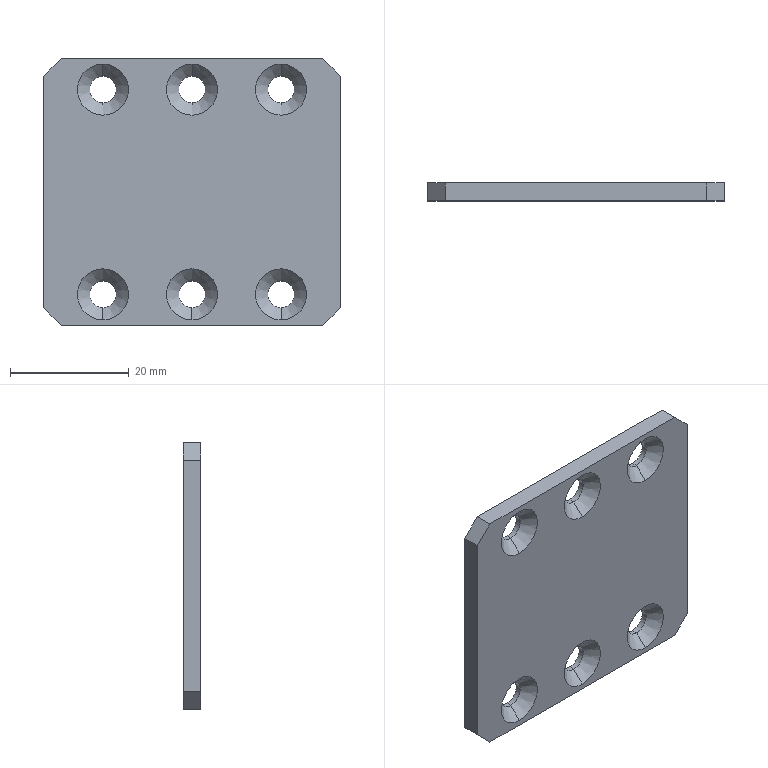Part | SolidWorks | features Chamfer 1, Extrusion 1, HoleWzd 1 | 1 solid | 34 faces | box 50 x 3 x 45 mm | volume 6177 mm3 | cone 12 | cylinder 12 | plane 10 | commonest cylinder face diameters 4.5 x12
STEP:
#1=CARTESIAN_POINT('',(-15.,2.05,-15.));
#2=VERTEX_POINT('',#1);
#3=CARTESIAN_POINT('',(-15.,2.05,-19.5));
#4=VERTEX_POINT('',#3);
#5=CARTESIAN_POINT('',(-15.,2.05,-17.25));
#6=DIRECTION('',(0.,-1.,0.));
#7=DIRECTION('',(0.,0.,-1.));
#8=AXIS2_PLACEMENT_3D('',#5,#6,#7);
#9=CIRCLE('',#8,2.25);
#10=EDGE_CURVE('',#2,#4,#9,.T.);
#11=ORIENTED_EDGE('',*,*,#10,.F.);
#12=CARTESIAN_POINT('',(-15.,0.,-12.95));
#13=VERTEX_POINT('',#12);
#14=CARTESIAN_POINT('',(-15.,0.,-12.95));
#15=DIRECTION('',(0.,-0.7071,0.7071));
#16=VECTOR('',#15,1000.);
#17=LINE('',#14,#16);
#18=EDGE_CURVE('',#2,#13,#17,.T.);
#19=ORIENTED_EDGE('',*,*,#18,.T.);
#20=CARTESIAN_POINT('',(-15.,0.,-21.55));
#21=VERTEX_POINT('',#20);
#22=CARTESIAN_POINT('',(-15.,0.,-17.25));
#23=DIRECTION('',(0.,-1.,0.));
#24=DIRECTION('',(0.,0.,-1.));
#25=AXIS2_PLACEMENT_3D('',#22,#23,#24);
#26=CIRCLE('',#25,4.3);
#27=EDGE_CURVE('',#13,#21,#26,.T.);
#28=ORIENTED_EDGE('',*,*,#27,.T.);
#29=CARTESIAN_POINT('',(-15.,0.,-21.55));
#30=DIRECTION('',(0.,-0.7071,-0.7071));
#31=VECTOR('',#30,1000.);
#32=LINE('',#29,#31);
#33=EDGE_CURVE('',#4,#21,#32,.T.);
#34=ORIENTED_EDGE('',*,*,#33,.F.);
#35=EDGE_LOOP('',(#11,#19,#28,#34));
#36=FACE_OUTER_BOUND('',#35,.T.);
#37=CARTESIAN_POINT('',(-15.,0.,-17.25));
#38=DIRECTION('',(0.,-1.,0.));
#39=DIRECTION('',(0.,0.,-1.));
#40=AXIS2_PLACEMENT_3D('',#37,#38,#39);
#41=CONICAL_SURFACE('',#40,4.3,0.7854);
#42=ADVANCED_FACE('',(#36),#41,.F.);
#43=CARTESIAN_POINT('',(-15.,3.,-19.5));
#44=VERTEX_POINT('',#43);
#45=CARTESIAN_POINT('',(-15.,3.,-15.));
#46=VERTEX_POINT('',#45);
#47=CARTESIAN_POINT('',(-15.,3.,-17.25));
#48=DIRECTION('',(0.,1.,0.));
#49=DIRECTION('',(0.,0.,1.));
#50=AXIS2_PLACEMENT_3D('',#47,#48,#49);
#51=CIRCLE('',#50,2.25);
#52=EDGE_CURVE('',#44,#46,#51,.T.);
#53=ORIENTED_EDGE('',*,*,#52,.T.);
#54=CARTESIAN_POINT('',(-15.,0.,-15.));
#55=DIRECTION('',(0.,-1.,0.));
#56=VECTOR('',#55,1000.);
#57=LINE('',#54,#56);
#58=EDGE_CURVE('',#46,#2,#57,.T.);
#59=ORIENTED_EDGE('',*,*,#58,.T.);
#60=ORIENTED_EDGE('',*,*,#10,.T.);
#61=CARTESIAN_POINT('',(-15.,0.,-19.5));
#62=DIRECTION('',(0.,-1.,0.));
#63=VECTOR('',#62,1000.);
#64=LINE('',#61,#63);
#65=EDGE_CURVE('',#44,#4,#64,.T.);
#66=ORIENTED_EDGE('',*,*,#65,.F.);
#67=EDGE_LOOP('',(#53,#59,#60,#66));
#68=FACE_OUTER_BOUND('',#67,.T.);
#69=CARTESIAN_POINT('',(-15.,0.,-17.25));
#70=DIRECTION('',(0.,-1.,0.));
#71=DIRECTION('',(0.,0.,-1.));
#72=AXIS2_PLACEMENT_3D('',#69,#70,#71);
#73=CYLINDRICAL_SURFACE('',#72,2.25);
#74=ADVANCED_FACE('',(#68),#73,.F.);
#75=CARTESIAN_POINT('',(0.,2.05,-15.));
#76=VERTEX_POINT('',#75);
#77=CARTESIAN_POINT('',(0.,2.05,-19.5));
#78=VERTEX_POINT('',#77);
#79=CARTESIAN_POINT('',(0.,2.05,-17.25));
#80=DIRECTION('',(0.,-1.,0.));
#81=DIRECTION('',(0.,0.,-1.));
#82=AXIS2_PLACEMENT_3D('',#79,#80,#81);
#83=CIRCLE('',#82,2.25);
#84=EDGE_CURVE('',#76,#78,#83,.T.);
#85=ORIENTED_EDGE('',*,*,#84,.F.);
#86=CARTESIAN_POINT('',(0.,0.,-12.95));
#87=VERTEX_POINT('',#86);
#88=CARTESIAN_POINT('',(0.,0.,-12.95));
#89=DIRECTION('',(0.,-0.7071,0.7071));
#90=VECTOR('',#89,1000.);
#91=LINE('',#88,#90);
#92=EDGE_CURVE('',#76,#87,#91,.T.);
#93=ORIENTED_EDGE('',*,*,#92,.T.);
#94=CARTESIAN_POINT('',(0.,0.,-21.55));
#95=VERTEX_POINT('',#94);
#96=CARTESIAN_POINT('',(0.,0.,-17.25));
#97=DIRECTION('',(0.,-1.,0.));
#98=DIRECTION('',(0.,0.,-1.));
#99=AXIS2_PLACEMENT_3D('',#96,#97,#98);
#100=CIRCLE('',#99,4.3);
#101=EDGE_CURVE('',#87,#95,#100,.T.);
#102=ORIENTED_EDGE('',*,*,#101,.T.);
#103=CARTESIAN_POINT('',(0.,0.,-21.55));
#104=DIRECTION('',(0.,-0.7071,-0.7071));
#105=VECTOR('',#104,1000.);
#106=LINE('',#103,#105);
#107=EDGE_CURVE('',#78,#95,#106,.T.);
#108=ORIENTED_EDGE('',*,*,#107,.F.);
#109=EDGE_LOOP('',(#85,#93,#102,#108));
#110=FACE_OUTER_BOUND('',#109,.T.);
#111=CARTESIAN_POINT('',(0.,0.,-17.25));
#112=DIRECTION('',(0.,-1.,0.));
#113=DIRECTION('',(0.,0.,-1.));
#114=AXIS2_PLACEMENT_3D('',#111,#112,#113);
#115=CONICAL_SURFACE('',#114,4.3,0.7854);
#116=ADVANCED_FACE('',(#110),#115,.F.);
#117=CARTESIAN_POINT('',(0.,3.,-19.5));
#118=VERTEX_POINT('',#117);
#119=CARTESIAN_POINT('',(0.,3.,-15.));
#120=VERTEX_POINT('',#119);
#121=CARTESIAN_POINT('',(0.,3.,-17.25));
#122=DIRECTION('',(0.,1.,0.));
#123=DIRECTION('',(0.,0.,1.));
#124=AXIS2_PLACEMENT_3D('',#121,#122,#123);
#125=CIRCLE('',#124,2.25);
#126=EDGE_CURVE('',#118,#120,#125,.T.);
#127=ORIENTED_EDGE('',*,*,#126,.T.);
#128=CARTESIAN_POINT('',(0.,0.,-15.));
#129=DIRECTION('',(0.,-1.,0.));
#130=VECTOR('',#129,1000.);
#131=LINE('',#128,#130);
#132=EDGE_CURVE('',#120,#76,#131,.T.);
#133=ORIENTED_EDGE('',*,*,#132,.T.);
#134=ORIENTED_EDGE('',*,*,#84,.T.);
#135=CARTESIAN_POINT('',(0.,0.,-19.5));
#136=DIRECTION('',(0.,-1.,0.));
#137=VECTOR('',#136,1000.);
#138=LINE('',#135,#137);
#139=EDGE_CURVE('',#118,#78,#138,.T.);
#140=ORIENTED_EDGE('',*,*,#139,.F.);
#141=EDGE_LOOP('',(#127,#133,#134,#140));
#142=FACE_OUTER_BOUND('',#141,.T.);
#143=CARTESIAN_POINT('',(0.,0.,-17.25));
#144=DIRECTION('',(0.,-1.,0.));
#145=DIRECTION('',(0.,0.,-1.));
#146=AXIS2_PLACEMENT_3D('',#143,#144,#145);
#147=CYLINDRICAL_SURFACE('',#146,2.25);
#148=ADVANCED_FACE('',(#142),#147,.F.);
#149=CARTESIAN_POINT('',(15.,2.05,-15.));
#150=VERTEX_POINT('',#149);
#151=CARTESIAN_POINT('',(15.,2.05,-19.5));
#152=VERTEX_POINT('',#151);
#153=CARTESIAN_POINT('',(15.,2.05,-17.25));
#154=DIRECTION('',(0.,-1.,0.));
#155=DIRECTION('',(0.,0.,-1.));
#156=AXIS2_PLACEMENT_3D('',#153,#154,#155);
#157=CIRCLE('',#156,2.25);
#158=EDGE_CURVE('',#150,#152,#157,.T.);
#159=ORIENTED_EDGE('',*,*,#158,.F.);
#160=CARTESIAN_POINT('',(15.,0.,-12.95));
#161=VERTEX_POINT('',#160);
#162=CARTESIAN_POINT('',(15.,0.,-12.95));
#163=DIRECTION('',(0.,-0.7071,0.7071));
#164=VECTOR('',#163,1000.);
#165=LINE('',#162,#164);
#166=EDGE_CURVE('',#150,#161,#165,.T.);
#167=ORIENTED_EDGE('',*,*,#166,.T.);
#168=CARTESIAN_POINT('',(15.,0.,-21.55));
#169=VERTEX_POINT('',#168);
#170=CARTESIAN_POINT('',(15.,0.,-17.25));
#171=DIRECTION('',(0.,-1.,0.));
#172=DIRECTION('',(0.,0.,-1.));
#173=AXIS2_PLACEMENT_3D('',#170,#171,#172);
#174=CIRCLE('',#173,4.3);
#175=EDGE_CURVE('',#161,#169,#174,.T.);
#176=ORIENTED_EDGE('',*,*,#175,.T.);
#177=CARTESIAN_POINT('',(15.,0.,-21.55));
#178=DIRECTION('',(0.,-0.7071,-0.7071));
#179=VECTOR('',#178,1000.);
#180=LINE('',#177,#179);
#181=EDGE_CURVE('',#152,#169,#180,.T.);
#182=ORIENTED_EDGE('',*,*,#181,.F.);
#183=EDGE_LOOP('',(#159,#167,#176,#182));
#184=FACE_OUTER_BOUND('',#183,.T.);
#185=CARTESIAN_POINT('',(15.,0.,-17.25));
#186=DIRECTION('',(0.,-1.,0.));
#187=DIRECTION('',(0.,0.,-1.));
#188=AXIS2_PLACEMENT_3D('',#185,#186,#187);
#189=CONICAL_SURFACE('',#188,4.3,0.7854);
#190=ADVANCED_FACE('',(#184),#189,.F.);
#191=CARTESIAN_POINT('',(15.,3.,-19.5));
#192=VERTEX_POINT('',#191);
#193=CARTESIAN_POINT('',(15.,3.,-15.));
#194=VERTEX_POINT('',#193);
#195=CARTESIAN_POINT('',(15.,3.,-17.25));
#196=DIRECTION('',(0.,1.,0.));
#197=DIRECTION('',(0.,0.,1.));
#198=AXIS2_PLACEMENT_3D('',#195,#196,#197);
#199=CIRCLE('',#198,2.25);
#200=EDGE_CURVE('',#192,#194,#199,.T.);
#201=ORIENTED_EDGE('',*,*,#200,.T.);
#202=CARTESIAN_POINT('',(15.,0.,-15.));
#203=DIRECTION('',(0.,-1.,0.));
#204=VECTOR('',#203,1000.);
#205=LINE('',#202,#204);
#206=EDGE_CURVE('',#194,#150,#205,.T.);
#207=ORIENTED_EDGE('',*,*,#206,.T.);
#208=ORIENTED_EDGE('',*,*,#158,.T.);
#209=CARTESIAN_POINT('',(15.,0.,-19.5));
#210=DIRECTION('',(0.,-1.,0.));
#211=VECTOR('',#210,1000.);
#212=LINE('',#209,#211);
#213=EDGE_CURVE('',#192,#152,#212,.T.);
#214=ORIENTED_EDGE('',*,*,#213,.F.);
#215=EDGE_LOOP('',(#201,#207,#208,#214));
#216=FACE_OUTER_BOUND('',#215,.T.);
#217=CARTESIAN_POINT('',(15.,0.,-17.25));
#218=DIRECTION('',(0.,-1.,0.));
#219=DIRECTION('',(0.,0.,-1.));
#220=AXIS2_PLACEMENT_3D('',#217,#218,#219);
#221=CYLINDRICAL_SURFACE('',#220,2.25);
#222=ADVANCED_FACE('',(#216),#221,.F.);
#223=CARTESIAN_POINT('',(15.,2.05,19.5));
#224=VERTEX_POINT('',#223);
#225=CARTESIAN_POINT('',(15.,2.05,15.));
#226=VERTEX_POINT('',#225);
#227=CARTESIAN_POINT('',(15.,2.05,17.25));
#228=DIRECTION('',(0.,-1.,0.));
#229=DIRECTION('',(0.,0.,-1.));
#230=AXIS2_PLACEMENT_3D('',#227,#228,#229);
#231=CIRCLE('',#230,2.25);
#232=EDGE_CURVE('',#224,#226,#231,.T.);
#233=ORIENTED_EDGE('',*,*,#232,.F.);
#234=CARTESIAN_POINT('',(15.,0.,21.55));
#235=VERTEX_POINT('',#234);
#236=CARTESIAN_POINT('',(15.,0.,21.55));
#237=DIRECTION('',(0.,-0.7071,0.7071));
#238=VECTOR('',#237,1000.);
#239=LINE('',#236,#238);
#240=EDGE_CURVE('',#224,#235,#239,.T.);
#241=ORIENTED_EDGE('',*,*,#240,.T.);
#242=CARTESIAN_POINT('',(15.,0.,12.95));
#243=VERTEX_POINT('',#242);
#244=CARTESIAN_POINT('',(15.,0.,17.25));
#245=DIRECTION('',(0.,-1.,0.));
#246=DIRECTION('',(0.,0.,-1.));
#247=AXIS2_PLACEMENT_3D('',#244,#245,#246);
#248=CIRCLE('',#247,4.3);
#249=EDGE_CURVE('',#235,#243,#248,.T.);
#250=ORIENTED_EDGE('',*,*,#249,.T.);
#251=CARTESIAN_POINT('',(15.,0.,12.95));
#252=DIRECTION('',(0.,-0.7071,-0.7071));
#253=VECTOR('',#252,1000.);
#254=LINE('',#251,#253);
#255=EDGE_CURVE('',#226,#243,#254,.T.);
#256=ORIENTED_EDGE('',*,*,#255,.F.);
#257=EDGE_LOOP('',(#233,#241,#250,#256));
#258=FACE_OUTER_BOUND('',#257,.T.);
#259=CARTESIAN_POINT('',(15.,0.,17.25));
#260=DIRECTION('',(0.,-1.,0.));
#261=DIRECTION('',(0.,0.,-1.));
#262=AXIS2_PLACEMENT_3D('',#259,#260,#261);
#263=CONICAL_SURFACE('',#262,4.3,0.7854);
#264=ADVANCED_FACE('',(#258),#263,.F.);
#265=CARTESIAN_POINT('',(15.,3.,15.));
#266=VERTEX_POINT('',#265);
#267=CARTESIAN_POINT('',(15.,3.,19.5));
#268=VERTEX_POINT('',#267);
#269=CARTESIAN_POINT('',(15.,3.,17.25));
#270=DIRECTION('',(0.,1.,0.));
#271=DIRECTION('',(0.,0.,1.));
#272=AXIS2_PLACEMENT_3D('',#269,#270,#271);
#273=CIRCLE('',#272,2.25);
#274=EDGE_CURVE('',#266,#268,#273,.T.);
#275=ORIENTED_EDGE('',*,*,#274,.T.);
#276=CARTESIAN_POINT('',(15.,0.,19.5));
#277=DIRECTION('',(0.,-1.,0.));
#278=VECTOR('',#277,1000.);
#279=LINE('',#276,#278);
#280=EDGE_CURVE('',#268,#224,#279,.T.);
#281=ORIENTED_EDGE('',*,*,#280,.T.);
#282=ORIENTED_EDGE('',*,*,#232,.T.);
#283=CARTESIAN_POINT('',(15.,0.,15.));
#284=DIRECTION('',(0.,-1.,0.));
#285=VECTOR('',#284,1000.);
#286=LINE('',#283,#285);
#287=EDGE_CURVE('',#266,#226,#286,.T.);
#288=ORIENTED_EDGE('',*,*,#287,.F.);
#289=EDGE_LOOP('',(#275,#281,#282,#288));
#290=FACE_OUTER_BOUND('',#289,.T.);
#291=CARTESIAN_POINT('',(15.,0.,17.25));
#292=DIRECTION('',(0.,-1.,0.));
#293=DIRECTION('',(0.,0.,-1.));
#294=AXIS2_PLACEMENT_3D('',#291,#292,#293);
#295=CYLINDRICAL_SURFACE('',#294,2.25);
#296=ADVANCED_FACE('',(#290),#295,.F.);
#297=CARTESIAN_POINT('',(0.,2.05,19.5));
#298=VERTEX_POINT('',#297);
#299=CARTESIAN_POINT('',(0.,2.05,15.));
#300=VERTEX_POINT('',#299);
#301=CARTESIAN_POINT('',(0.,2.05,17.25));
#302=DIRECTION('',(0.,-1.,0.));
#303=DIRECTION('',(0.,0.,-1.));
#304=AXIS2_PLACEMENT_3D('',#301,#302,#303);
#305=CIRCLE('',#304,2.25);
#306=EDGE_CURVE('',#298,#300,#305,.T.);
#307=ORIENTED_EDGE('',*,*,#306,.F.);
#308=CARTESIAN_POINT('',(0.,0.,21.55));
#309=VERTEX_POINT('',#308);
#310=CARTESIAN_POINT('',(0.,0.,21.55));
#311=DIRECTION('',(0.,-0.7071,0.7071));
#312=VECTOR('',#311,1000.);
#313=LINE('',#310,#312);
#314=EDGE_CURVE('',#298,#309,#313,.T.);
#315=ORIENTED_EDGE('',*,*,#314,.T.);
#316=CARTESIAN_POINT('',(0.,0.,12.95));
#317=VERTEX_POINT('',#316);
#318=CARTESIAN_POINT('',(0.,0.,17.25));
#319=DIRECTION('',(0.,-1.,0.));
#320=DIRECTION('',(0.,0.,-1.));
#321=AXIS2_PLACEMENT_3D('',#318,#319,#320);
#322=CIRCLE('',#321,4.3);
#323=EDGE_CURVE('',#309,#317,#322,.T.);
#324=ORIENTED_EDGE('',*,*,#323,.T.);
#325=CARTESIAN_POINT('',(0.,0.,12.95));
#326=DIRECTION('',(0.,-0.7071,-0.7071));
#327=VECTOR('',#326,1000.);
#328=LINE('',#325,#327);
#329=EDGE_CURVE('',#300,#317,#328,.T.);
#330=ORIENTED_EDGE('',*,*,#329,.F.);
#331=EDGE_LOOP('',(#307,#315,#324,#330));
#332=FACE_OUTER_BOUND('',#331,.T.);
#333=CARTESIAN_POINT('',(0.,0.,17.25));
#334=DIRECTION('',(0.,-1.,0.));
#335=DIRECTION('',(0.,0.,-1.));
#336=AXIS2_PLACEMENT_3D('',#333,#334,#335);
#337=CONICAL_SURFACE('',#336,4.3,0.7854);
#338=ADVANCED_FACE('',(#332),#337,.F.);
#339=CARTESIAN_POINT('',(0.,3.,15.));
#340=VERTEX_POINT('',#339);
#341=CARTESIAN_POINT('',(0.,3.,19.5));
#342=VERTEX_POINT('',#341);
#343=CARTESIAN_POINT('',(0.,3.,17.25));
#344=DIRECTION('',(0.,1.,0.));
#345=DIRECTION('',(0.,0.,1.));
#346=AXIS2_PLACEMENT_3D('',#343,#344,#345);
#347=CIRCLE('',#346,2.25);
#348=EDGE_CURVE('',#340,#342,#347,.T.);
#349=ORIENTED_EDGE('',*,*,#348,.T.);
#350=CARTESIAN_POINT('',(0.,0.,19.5));
#351=DIRECTION('',(0.,-1.,0.));
#352=VECTOR('',#351,1000.);
#353=LINE('',#350,#352);
#354=EDGE_CURVE('',#342,#298,#353,.T.);
#355=ORIENTED_EDGE('',*,*,#354,.T.);
#356=ORIENTED_EDGE('',*,*,#306,.T.);
#357=CARTESIAN_POINT('',(0.,0.,15.));
#358=DIRECTION('',(0.,-1.,0.));
#359=VECTOR('',#358,1000.);
#360=LINE('',#357,#359);
#361=EDGE_CURVE('',#340,#300,#360,.T.);
#362=ORIENTED_EDGE('',*,*,#361,.F.);
#363=EDGE_LOOP('',(#349,#355,#356,#362));
#364=FACE_OUTER_BOUND('',#363,.T.);
#365=CARTESIAN_POINT('',(0.,0.,17.25));
#366=DIRECTION('',(0.,-1.,0.));
#367=DIRECTION('',(0.,0.,-1.));
#368=AXIS2_PLACEMENT_3D('',#365,#366,#367);
#369=CYLINDRICAL_SURFACE('',#368,2.25);
#370=ADVANCED_FACE('',(#364),#369,.F.);
#371=CARTESIAN_POINT('',(-15.,2.05,19.5));
#372=VERTEX_POINT('',#371);
#373=CARTESIAN_POINT('',(-15.,2.05,15.));
#374=VERTEX_POINT('',#373);
#375=CARTESIAN_POINT('',(-15.,2.05,17.25));
#376=DIRECTION('',(0.,-1.,0.));
#377=DIRECTION('',(0.,0.,-1.));
#378=AXIS2_PLACEMENT_3D('',#375,#376,#377);
#379=CIRCLE('',#378,2.25);
#380=EDGE_CURVE('',#372,#374,#379,.T.);
#381=ORIENTED_EDGE('',*,*,#380,.F.);
#382=CARTESIAN_POINT('',(-15.,0.,21.55));
#383=VERTEX_POINT('',#382);
#384=CARTESIAN_POINT('',(-15.,0.,21.55));
#385=DIRECTION('',(0.,-0.7071,0.7071));
#386=VECTOR('',#385,1000.);
#387=LINE('',#384,#386);
#388=EDGE_CURVE('',#372,#383,#387,.T.);
#389=ORIENTED_EDGE('',*,*,#388,.T.);
#390=CARTESIAN_POINT('',(-15.,0.,12.95));
#391=VERTEX_POINT('',#390);
#392=CARTESIAN_POINT('',(-15.,0.,17.25));
#393=DIRECTION('',(0.,-1.,0.));
#394=DIRECTION('',(0.,0.,-1.));
#395=AXIS2_PLACEMENT_3D('',#392,#393,#394);
#396=CIRCLE('',#395,4.3);
#397=EDGE_CURVE('',#383,#391,#396,.T.);
#398=ORIENTED_EDGE('',*,*,#397,.T.);
#399=CARTESIAN_POINT('',(-15.,0.,12.95));
#400=DIRECTION('',(0.,-0.7071,-0.7071));
#401=VECTOR('',#400,1000.);
#402=LINE('',#399,#401);
#403=EDGE_CURVE('',#374,#391,#402,.T.);
#404=ORIENTED_EDGE('',*,*,#403,.F.);
#405=EDGE_LOOP('',(#381,#389,#398,#404));
#406=FACE_OUTER_BOUND('',#405,.T.);
#407=CARTESIAN_POINT('',(-15.,0.,17.25));
#408=DIRECTION('',(0.,-1.,0.));
#409=DIRECTION('',(0.,0.,-1.));
#410=AXIS2_PLACEMENT_3D('',#407,#408,#409);
#411=CONICAL_SURFACE('',#410,4.3,0.7854);
#412=ADVANCED_FACE('',(#406),#411,.F.);
#413=CARTESIAN_POINT('',(-15.,3.,15.));
#414=VERTEX_POINT('',#413);
#415=CARTESIAN_POINT('',(-15.,3.,19.5));
#416=VERTEX_POINT('',#415);
#417=CARTESIAN_POINT('',(-15.,3.,17.25));
#418=DIRECTION('',(0.,1.,0.));
#419=DIRECTION('',(0.,0.,1.));
#420=AXIS2_PLACEMENT_3D('',#417,#418,#419);
#421=CIRCLE('',#420,2.25);
#422=EDGE_CURVE('',#414,#416,#421,.T.);
#423=ORIENTED_EDGE('',*,*,#422,.T.);
#424=CARTESIAN_POINT('',(-15.,0.,19.5));
#425=DIRECTION('',(0.,-1.,0.));
#426=VECTOR('',#425,1000.);
#427=LINE('',#424,#426);
#428=EDGE_CURVE('',#416,#372,#427,.T.);
#429=ORIENTED_EDGE('',*,*,#428,.T.);
#430=ORIENTED_EDGE('',*,*,#380,.T.);
#431=CARTESIAN_POINT('',(-15.,0.,15.));
#432=DIRECTION('',(0.,-1.,0.));
#433=VECTOR('',#432,1000.);
#434=LINE('',#431,#433);
#435=EDGE_CURVE('',#414,#374,#434,.T.);
#436=ORIENTED_EDGE('',*,*,#435,.F.);
#437=EDGE_LOOP('',(#423,#429,#430,#436));
#438=FACE_OUTER_BOUND('',#437,.T.);
#439=CARTESIAN_POINT('',(-15.,0.,17.25));
#440=DIRECTION('',(0.,-1.,0.));
#441=DIRECTION('',(0.,0.,-1.));
#442=AXIS2_PLACEMENT_3D('',#439,#440,#441);
#443=CYLINDRICAL_SURFACE('',#442,2.25);
#444=ADVANCED_FACE('',(#438),#443,.F.);
#445=CARTESIAN_POINT('',(25.,0.,19.5));
#446=VERTEX_POINT('',#445);
#447=CARTESIAN_POINT('',(25.,0.,-19.5));
#448=VERTEX_POINT('',#447);
#449=CARTESIAN_POINT('',(25.,0.,-22.5));
#450=DIRECTION('',(0.,0.,-1.));
#451=VECTOR('',#450,1000.);
#452=LINE('',#449,#451);
#453=EDGE_CURVE('',#446,#448,#452,.T.);
#454=ORIENTED_EDGE('',*,*,#453,.T.);
#455=CARTESIAN_POINT('',(25.,3.,-19.5));
#456=VERTEX_POINT('',#455);
#457=CARTESIAN_POINT('',(25.,3.,-19.5));
#458=DIRECTION('',(0.,1.,0.));
#459=VECTOR('',#458,1000.);
#460=LINE('',#457,#459);
#461=EDGE_CURVE('',#448,#456,#460,.T.);
#462=ORIENTED_EDGE('',*,*,#461,.T.);
#463=CARTESIAN_POINT('',(25.,3.,19.5));
#464=VERTEX_POINT('',#463);
#465=CARTESIAN_POINT('',(25.,3.,-22.5));
#466=DIRECTION('',(0.,0.,-1.));
#467=VECTOR('',#466,1000.);
#468=LINE('',#465,#467);
#469=EDGE_CURVE('',#464,#456,#468,.T.);
#470=ORIENTED_EDGE('',*,*,#469,.F.);
#471=CARTESIAN_POINT('',(25.,3.,19.5));
#472=DIRECTION('',(0.,-1.,0.));
#473=VECTOR('',#472,1000.);
#474=LINE('',#471,#473);
#475=EDGE_CURVE('',#464,#446,#474,.T.);
#476=ORIENTED_EDGE('',*,*,#475,.T.);
#477=EDGE_LOOP('',(#454,#462,#470,#476));
#478=FACE_OUTER_BOUND('',#477,.T.);
#479=CARTESIAN_POINT('',(25.,3.,-22.5));
#480=DIRECTION('',(-1.,0.,0.));
#481=DIRECTION('',(0.,0.,1.));
#482=AXIS2_PLACEMENT_3D('',#479,#480,#481);
#483=PLANE('',#482);
#484=ADVANCED_FACE('',(#478),#483,.F.);
#485=CARTESIAN_POINT('',(22.,0.,-22.5));
#486=VERTEX_POINT('',#485);
#487=CARTESIAN_POINT('',(-22.,0.,-22.5));
#488=VERTEX_POINT('',#487);
#489=CARTESIAN_POINT('',(-25.,0.,-22.5));
#490=DIRECTION('',(-1.,0.,0.));
#491=VECTOR('',#490,1000.);
#492=LINE('',#489,#491);
#493=EDGE_CURVE('',#486,#488,#492,.T.);
#494=ORIENTED_EDGE('',*,*,#493,.T.);
#495=CARTESIAN_POINT('',(-22.,3.,-22.5));
#496=VERTEX_POINT('',#495);
#497=CARTESIAN_POINT('',(-22.,3.,-22.5));
#498=DIRECTION('',(0.,1.,0.));
#499=VECTOR('',#498,1000.);
#500=LINE('',#497,#499);
#501=EDGE_CURVE('',#488,#496,#500,.T.);
#502=ORIENTED_EDGE('',*,*,#501,.T.);
#503=CARTESIAN_POINT('',(22.,3.,-22.5));
#504=VERTEX_POINT('',#503);
#505=CARTESIAN_POINT('',(-25.,3.,-22.5));
#506=DIRECTION('',(-1.,0.,0.));
#507=VECTOR('',#506,1000.);
#508=LINE('',#505,#507);
#509=EDGE_CURVE('',#504,#496,#508,.T.);
#510=ORIENTED_EDGE('',*,*,#509,.F.);
#511=CARTESIAN_POINT('',(22.,3.,-22.5));
#512=DIRECTION('',(0.,-1.,0.));
#513=VECTOR('',#512,1000.);
#514=LINE('',#511,#513);
#515=EDGE_CURVE('',#504,#486,#514,.T.);
#516=ORIENTED_EDGE('',*,*,#515,.T.);
#517=EDGE_LOOP('',(#494,#502,#510,#516));
#518=FACE_OUTER_BOUND('',#517,.T.);
#519=CARTESIAN_POINT('',(-25.,3.,-22.5));
#520=DIRECTION('',(0.,0.,1.));
#521=DIRECTION('',(1.,0.,0.));
#522=AXIS2_PLACEMENT_3D('',#519,#520,#521);
#523=PLANE('',#522);
#524=ADVANCED_FACE('',(#518),#523,.F.);
#525=CARTESIAN_POINT('',(-25.,3.,-19.5));
#526=VERTEX_POINT('',#525);
#527=CARTESIAN_POINT('',(-25.,3.,19.5));
#528=VERTEX_POINT('',#527);
#529=CARTESIAN_POINT('',(-25.,3.,-22.5));
#530=DIRECTION('',(0.,0.,1.));
#531=VECTOR('',#530,1000.);
#532=LINE('',#529,#531);
#533=EDGE_CURVE('',#526,#528,#532,.T.);
#534=ORIENTED_EDGE('',*,*,#533,.F.);
#535=CARTESIAN_POINT('',(-25.,0.,-19.5));
#536=VERTEX_POINT('',#535);
#537=CARTESIAN_POINT('',(-25.,3.,-19.5));
#538=DIRECTION('',(0.,-1.,0.));
#539=VECTOR('',#538,1000.);
#540=LINE('',#537,#539);
#541=EDGE_CURVE('',#526,#536,#540,.T.);
#542=ORIENTED_EDGE('',*,*,#541,.T.);
#543=CARTESIAN_POINT('',(-25.,0.,19.5));
#544=VERTEX_POINT('',#543);
#545=CARTESIAN_POINT('',(-25.,0.,-22.5));
#546=DIRECTION('',(0.,0.,1.));
#547=VECTOR('',#546,1000.);
#548=LINE('',#545,#547);
#549=EDGE_CURVE('',#536,#544,#548,.T.);
#550=ORIENTED_EDGE('',*,*,#549,.T.);
#551=CARTESIAN_POINT('',(-25.,3.,19.5));
#552=DIRECTION('',(0.,1.,0.));
#553=VECTOR('',#552,1000.);
#554=LINE('',#551,#553);
#555=EDGE_CURVE('',#544,#528,#554,.T.);
#556=ORIENTED_EDGE('',*,*,#555,.T.);
#557=EDGE_LOOP('',(#534,#542,#550,#556));
#558=FACE_OUTER_BOUND('',#557,.T.);
#559=CARTESIAN_POINT('',(-25.,3.,-22.5));
#560=DIRECTION('',(1.,0.,0.));
#561=DIRECTION('',(0.,0.,-1.));
#562=AXIS2_PLACEMENT_3D('',#559,#560,#561);
#563=PLANE('',#562);
#564=ADVANCED_FACE('',(#558),#563,.F.);
#565=CARTESIAN_POINT('',(-22.,0.,22.5));
#566=VERTEX_POINT('',#565);
#567=CARTESIAN_POINT('',(22.,0.,22.5));
#568=VERTEX_POINT('',#567);
#569=CARTESIAN_POINT('',(-25.,0.,22.5));
#570=DIRECTION('',(1.,0.,0.));
#571=VECTOR('',#570,1000.);
#572=LINE('',#569,#571);
#573=EDGE_CURVE('',#566,#568,#572,.T.);
#574=ORIENTED_EDGE('',*,*,#573,.T.);
#575=CARTESIAN_POINT('',(22.,3.,22.5));
#576=VERTEX_POINT('',#575);
#577=CARTESIAN_POINT('',(22.,3.,22.5));
#578=DIRECTION('',(0.,1.,0.));
#579=VECTOR('',#578,1000.);
#580=LINE('',#577,#579);
#581=EDGE_CURVE('',#568,#576,#580,.T.);
#582=ORIENTED_EDGE('',*,*,#581,.T.);
#583=CARTESIAN_POINT('',(-22.,3.,22.5));
#584=VERTEX_POINT('',#583);
#585=CARTESIAN_POINT('',(-25.,3.,22.5));
#586=DIRECTION('',(1.,0.,0.));
#587=VECTOR('',#586,1000.);
#588=LINE('',#585,#587);
#589=EDGE_CURVE('',#584,#576,#588,.T.);
#590=ORIENTED_EDGE('',*,*,#589,.F.);
#591=CARTESIAN_POINT('',(-22.,3.,22.5));
#592=DIRECTION('',(0.,-1.,0.));
#593=VECTOR('',#592,1000.);
#594=LINE('',#591,#593);
#595=EDGE_CURVE('',#584,#566,#594,.T.);
#596=ORIENTED_EDGE('',*,*,#595,.T.);
#597=EDGE_LOOP('',(#574,#582,#590,#596));
#598=FACE_OUTER_BOUND('',#597,.T.);
#599=CARTESIAN_POINT('',(-25.,3.,22.5));
#600=DIRECTION('',(0.,0.,-1.));
#601=DIRECTION('',(-1.,0.,0.));
#602=AXIS2_PLACEMENT_3D('',#599,#600,#601);
#603=PLANE('',#602);
#604=ADVANCED_FACE('',(#598),#603,.F.);
#605=ORIENTED_EDGE('',*,*,#52,.F.);
#606=CARTESIAN_POINT('',(-15.,3.,-17.25));
#607=DIRECTION('',(0.,1.,0.));
#608=DIRECTION('',(0.,0.,1.));
#609=AXIS2_PLACEMENT_3D('',#606,#607,#608);
#610=CIRCLE('',#609,2.25);
#611=EDGE_CURVE('',#46,#44,#610,.T.);
#612=ORIENTED_EDGE('',*,*,#611,.F.);
#613=EDGE_LOOP('',(#605,#612));
#614=FACE_BOUND('',#613,.T.);
#615=ORIENTED_EDGE('',*,*,#126,.F.);
#616=CARTESIAN_POINT('',(0.,3.,-17.25));
#617=DIRECTION('',(0.,1.,0.));
#618=DIRECTION('',(0.,0.,1.));
#619=AXIS2_PLACEMENT_3D('',#616,#617,#618);
#620=CIRCLE('',#619,2.25);
#621=EDGE_CURVE('',#120,#118,#620,.T.);
#622=ORIENTED_EDGE('',*,*,#621,.F.);
#623=EDGE_LOOP('',(#615,#622));
#624=FACE_BOUND('',#623,.T.);
#625=ORIENTED_EDGE('',*,*,#200,.F.);
#626=CARTESIAN_POINT('',(15.,3.,-17.25));
#627=DIRECTION('',(0.,1.,0.));
#628=DIRECTION('',(0.,0.,1.));
#629=AXIS2_PLACEMENT_3D('',#626,#627,#628);
#630=CIRCLE('',#629,2.25);
#631=EDGE_CURVE('',#194,#192,#630,.T.);
#632=ORIENTED_EDGE('',*,*,#631,.F.);
#633=EDGE_LOOP('',(#625,#632));
#634=FACE_BOUND('',#633,.T.);
#635=ORIENTED_EDGE('',*,*,#274,.F.);
#636=CARTESIAN_POINT('',(15.,3.,17.25));
#637=DIRECTION('',(0.,1.,0.));
#638=DIRECTION('',(0.,0.,1.));
#639=AXIS2_PLACEMENT_3D('',#636,#637,#638);
#640=CIRCLE('',#639,2.25);
#641=EDGE_CURVE('',#268,#266,#640,.T.);
#642=ORIENTED_EDGE('',*,*,#641,.F.);
#643=EDGE_LOOP('',(#635,#642));
#644=FACE_BOUND('',#643,.T.);
#645=ORIENTED_EDGE('',*,*,#348,.F.);
#646=CARTESIAN_POINT('',(0.,3.,17.25));
#647=DIRECTION('',(0.,1.,0.));
#648=DIRECTION('',(0.,0.,1.));
#649=AXIS2_PLACEMENT_3D('',#646,#647,#648);
#650=CIRCLE('',#649,2.25);
#651=EDGE_CURVE('',#342,#340,#650,.T.);
#652=ORIENTED_EDGE('',*,*,#651,.F.);
#653=EDGE_LOOP('',(#645,#652));
#654=FACE_BOUND('',#653,.T.);
#655=ORIENTED_EDGE('',*,*,#422,.F.);
#656=CARTESIAN_POINT('',(-15.,3.,17.25));
#657=DIRECTION('',(0.,1.,0.));
#658=DIRECTION('',(0.,0.,1.));
#659=AXIS2_PLACEMENT_3D('',#656,#657,#658);
#660=CIRCLE('',#659,2.25);
#661=EDGE_CURVE('',#416,#414,#660,.T.);
#662=ORIENTED_EDGE('',*,*,#661,.F.);
#663=EDGE_LOOP('',(#655,#662));
#664=FACE_BOUND('',#663,.T.);
#665=ORIENTED_EDGE('',*,*,#509,.T.);
#666=CARTESIAN_POINT('',(-22.25,3.,-22.25));
#667=DIRECTION('',(-0.7071,0.,0.7071));
#668=VECTOR('',#667,1000.);
#669=LINE('',#666,#668);
#670=EDGE_CURVE('',#496,#526,#669,.T.);
#671=ORIENTED_EDGE('',*,*,#670,.T.);
#672=ORIENTED_EDGE('',*,*,#533,.T.);
#673=CARTESIAN_POINT('',(-22.25,3.,22.25));
#674=DIRECTION('',(0.7071,0.,0.7071));
#675=VECTOR('',#674,1000.);
#676=LINE('',#673,#675);
#677=EDGE_CURVE('',#528,#584,#676,.T.);
#678=ORIENTED_EDGE('',*,*,#677,.T.);
#679=ORIENTED_EDGE('',*,*,#589,.T.);
#680=CARTESIAN_POINT('',(22.25,3.,22.25));
#681=DIRECTION('',(0.7071,0.,-0.7071));
#682=VECTOR('',#681,1000.);
#683=LINE('',#680,#682);
#684=EDGE_CURVE('',#576,#464,#683,.T.);
#685=ORIENTED_EDGE('',*,*,#684,.T.);
#686=ORIENTED_EDGE('',*,*,#469,.T.);
#687=CARTESIAN_POINT('',(22.25,3.,-22.25));
#688=DIRECTION('',(-0.7071,0.,-0.7071));
#689=VECTOR('',#688,1000.);
#690=LINE('',#687,#689);
#691=EDGE_CURVE('',#456,#504,#690,.T.);
#692=ORIENTED_EDGE('',*,*,#691,.T.);
#693=EDGE_LOOP('',(#665,#671,#672,#678,#679,#685,#686,#692));
#694=FACE_OUTER_BOUND('',#693,.T.);
#695=CARTESIAN_POINT('',(0.,3.,0.));
#696=DIRECTION('',(0.,1.,0.));
#697=DIRECTION('',(0.,0.,1.));
#698=AXIS2_PLACEMENT_3D('',#695,#696,#697);
#699=PLANE('',#698);
#700=ADVANCED_FACE('',(#614,#624,#634,#644,#654,#664,#694),#699,.T.);
#701=CARTESIAN_POINT('',(-15.,0.,-17.25));
#702=DIRECTION('',(0.,-1.,0.));
#703=DIRECTION('',(0.,0.,-1.));
#704=AXIS2_PLACEMENT_3D('',#701,#702,#703);
#705=CIRCLE('',#704,4.3);
#706=EDGE_CURVE('',#21,#13,#705,.T.);
#707=ORIENTED_EDGE('',*,*,#706,.F.);
#708=ORIENTED_EDGE('',*,*,#27,.F.);
#709=EDGE_LOOP('',(#707,#708));
#710=FACE_BOUND('',#709,.T.);
#711=CARTESIAN_POINT('',(0.,0.,-17.25));
#712=DIRECTION('',(0.,-1.,0.));
#713=DIRECTION('',(0.,0.,-1.));
#714=AXIS2_PLACEMENT_3D('',#711,#712,#713);
#715=CIRCLE('',#714,4.3);
#716=EDGE_CURVE('',#95,#87,#715,.T.);
#717=ORIENTED_EDGE('',*,*,#716,.F.);
#718=ORIENTED_EDGE('',*,*,#101,.F.);
#719=EDGE_LOOP('',(#717,#718));
#720=FACE_BOUND('',#719,.T.);
#721=CARTESIAN_POINT('',(15.,0.,-17.25));
#722=DIRECTION('',(0.,-1.,0.));
#723=DIRECTION('',(0.,0.,-1.));
#724=AXIS2_PLACEMENT_3D('',#721,#722,#723);
#725=CIRCLE('',#724,4.3);
#726=EDGE_CURVE('',#169,#161,#725,.T.);
#727=ORIENTED_EDGE('',*,*,#726,.F.);
#728=ORIENTED_EDGE('',*,*,#175,.F.);
#729=EDGE_LOOP('',(#727,#728));
#730=FACE_BOUND('',#729,.T.);
#731=CARTESIAN_POINT('',(15.,0.,17.25));
#732=DIRECTION('',(0.,-1.,0.));
#733=DIRECTION('',(0.,0.,-1.));
#734=AXIS2_PLACEMENT_3D('',#731,#732,#733);
#735=CIRCLE('',#734,4.3);
#736=EDGE_CURVE('',#243,#235,#735,.T.);
#737=ORIENTED_EDGE('',*,*,#736,.F.);
#738=ORIENTED_EDGE('',*,*,#249,.F.);
#739=EDGE_LOOP('',(#737,#738));
#740=FACE_BOUND('',#739,.T.);
#741=CARTESIAN_POINT('',(0.,0.,17.25));
#742=DIRECTION('',(0.,-1.,0.));
#743=DIRECTION('',(0.,0.,-1.));
#744=AXIS2_PLACEMENT_3D('',#741,#742,#743);
#745=CIRCLE('',#744,4.3);
#746=EDGE_CURVE('',#317,#309,#745,.T.);
#747=ORIENTED_EDGE('',*,*,#746,.F.);
#748=ORIENTED_EDGE('',*,*,#323,.F.);
#749=EDGE_LOOP('',(#747,#748));
#750=FACE_BOUND('',#749,.T.);
#751=CARTESIAN_POINT('',(-15.,0.,17.25));
#752=DIRECTION('',(0.,-1.,0.));
#753=DIRECTION('',(0.,0.,-1.));
#754=AXIS2_PLACEMENT_3D('',#751,#752,#753);
#755=CIRCLE('',#754,4.3);
#756=EDGE_CURVE('',#391,#383,#755,.T.);
#757=ORIENTED_EDGE('',*,*,#756,.F.);
#758=ORIENTED_EDGE('',*,*,#397,.F.);
#759=EDGE_LOOP('',(#757,#758));
#760=FACE_BOUND('',#759,.T.);
#761=ORIENTED_EDGE('',*,*,#549,.F.);
#762=CARTESIAN_POINT('',(-25.,0.,-19.5));
#763=DIRECTION('',(0.7071,0.,-0.7071));
#764=VECTOR('',#763,1000.);
#765=LINE('',#762,#764);
#766=EDGE_CURVE('',#536,#488,#765,.T.);
#767=ORIENTED_EDGE('',*,*,#766,.T.);
#768=ORIENTED_EDGE('',*,*,#493,.F.);
#769=CARTESIAN_POINT('',(22.,0.,-22.5));
#770=DIRECTION('',(0.7071,0.,0.7071));
#771=VECTOR('',#770,1000.);
#772=LINE('',#769,#771);
#773=EDGE_CURVE('',#486,#448,#772,.T.);
#774=ORIENTED_EDGE('',*,*,#773,.T.);
#775=ORIENTED_EDGE('',*,*,#453,.F.);
#776=CARTESIAN_POINT('',(25.,0.,19.5));
#777=DIRECTION('',(-0.7071,0.,0.7071));
#778=VECTOR('',#777,1000.);
#779=LINE('',#776,#778);
#780=EDGE_CURVE('',#446,#568,#779,.T.);
#781=ORIENTED_EDGE('',*,*,#780,.T.);
#782=ORIENTED_EDGE('',*,*,#573,.F.);
#783=CARTESIAN_POINT('',(-22.,0.,22.5));
#784=DIRECTION('',(-0.7071,0.,-0.7071));
#785=VECTOR('',#784,1000.);
#786=LINE('',#783,#785);
#787=EDGE_CURVE('',#566,#544,#786,.T.);
#788=ORIENTED_EDGE('',*,*,#787,.T.);
#789=EDGE_LOOP('',(#761,#767,#768,#774,#775,#781,#782,#788));
#790=FACE_OUTER_BOUND('',#789,.T.);
#791=CARTESIAN_POINT('',(0.,0.,0.));
#792=DIRECTION('',(0.,1.,0.));
#793=DIRECTION('',(0.,0.,1.));
#794=AXIS2_PLACEMENT_3D('',#791,#792,#793);
#795=PLANE('',#794);
#796=ADVANCED_FACE('',(#710,#720,#730,#740,#750,#760,#790),#795,.F.);
#797=ORIENTED_EDGE('',*,*,#428,.F.);
#798=ORIENTED_EDGE('',*,*,#661,.T.);
#799=ORIENTED_EDGE('',*,*,#435,.T.);
#800=CARTESIAN_POINT('',(-15.,2.05,17.25));
#801=DIRECTION('',(0.,-1.,0.));
#802=DIRECTION('',(0.,0.,-1.));
#803=AXIS2_PLACEMENT_3D('',#800,#801,#802);
#804=CIRCLE('',#803,2.25);
#805=EDGE_CURVE('',#374,#372,#804,.T.);
#806=ORIENTED_EDGE('',*,*,#805,.T.);
#807=EDGE_LOOP('',(#797,#798,#799,#806));
#808=FACE_OUTER_BOUND('',#807,.T.);
#809=CARTESIAN_POINT('',(-15.,0.,17.25));
#810=DIRECTION('',(0.,-1.,0.));
#811=DIRECTION('',(0.,0.,-1.));
#812=AXIS2_PLACEMENT_3D('',#809,#810,#811);
#813=CYLINDRICAL_SURFACE('',#812,2.25);
#814=ADVANCED_FACE('',(#808),#813,.F.);
#815=ORIENTED_EDGE('',*,*,#388,.F.);
#816=ORIENTED_EDGE('',*,*,#805,.F.);
#817=ORIENTED_EDGE('',*,*,#403,.T.);
#818=ORIENTED_EDGE('',*,*,#756,.T.);
#819=EDGE_LOOP('',(#815,#816,#817,#818));
#820=FACE_OUTER_BOUND('',#819,.T.);
#821=CARTESIAN_POINT('',(-15.,0.,17.25));
#822=DIRECTION('',(0.,-1.,0.));
#823=DIRECTION('',(0.,0.,-1.));
#824=AXIS2_PLACEMENT_3D('',#821,#822,#823);
#825=CONICAL_SURFACE('',#824,4.3,0.7854);
#826=ADVANCED_FACE('',(#820),#825,.F.);
#827=ORIENTED_EDGE('',*,*,#354,.F.);
#828=ORIENTED_EDGE('',*,*,#651,.T.);
#829=ORIENTED_EDGE('',*,*,#361,.T.);
#830=CARTESIAN_POINT('',(0.,2.05,17.25));
#831=DIRECTION('',(0.,-1.,0.));
#832=DIRECTION('',(0.,0.,-1.));
#833=AXIS2_PLACEMENT_3D('',#830,#831,#832);
#834=CIRCLE('',#833,2.25);
#835=EDGE_CURVE('',#300,#298,#834,.T.);
#836=ORIENTED_EDGE('',*,*,#835,.T.);
#837=EDGE_LOOP('',(#827,#828,#829,#836));
#838=FACE_OUTER_BOUND('',#837,.T.);
#839=CARTESIAN_POINT('',(0.,0.,17.25));
#840=DIRECTION('',(0.,-1.,0.));
#841=DIRECTION('',(0.,0.,-1.));
#842=AXIS2_PLACEMENT_3D('',#839,#840,#841);
#843=CYLINDRICAL_SURFACE('',#842,2.25);
#844=ADVANCED_FACE('',(#838),#843,.F.);
#845=ORIENTED_EDGE('',*,*,#314,.F.);
#846=ORIENTED_EDGE('',*,*,#835,.F.);
#847=ORIENTED_EDGE('',*,*,#329,.T.);
#848=ORIENTED_EDGE('',*,*,#746,.T.);
#849=EDGE_LOOP('',(#845,#846,#847,#848));
#850=FACE_OUTER_BOUND('',#849,.T.);
#851=CARTESIAN_POINT('',(0.,0.,17.25));
#852=DIRECTION('',(0.,-1.,0.));
#853=DIRECTION('',(0.,0.,-1.));
#854=AXIS2_PLACEMENT_3D('',#851,#852,#853);
#855=CONICAL_SURFACE('',#854,4.3,0.7854);
#856=ADVANCED_FACE('',(#850),#855,.F.);
#857=ORIENTED_EDGE('',*,*,#280,.F.);
#858=ORIENTED_EDGE('',*,*,#641,.T.);
#859=ORIENTED_EDGE('',*,*,#287,.T.);
#860=CARTESIAN_POINT('',(15.,2.05,17.25));
#861=DIRECTION('',(0.,-1.,0.));
#862=DIRECTION('',(0.,0.,-1.));
#863=AXIS2_PLACEMENT_3D('',#860,#861,#862);
#864=CIRCLE('',#863,2.25);
#865=EDGE_CURVE('',#226,#224,#864,.T.);
#866=ORIENTED_EDGE('',*,*,#865,.T.);
#867=EDGE_LOOP('',(#857,#858,#859,#866));
#868=FACE_OUTER_BOUND('',#867,.T.);
#869=CARTESIAN_POINT('',(15.,0.,17.25));
#870=DIRECTION('',(0.,-1.,0.));
#871=DIRECTION('',(0.,0.,-1.));
#872=AXIS2_PLACEMENT_3D('',#869,#870,#871);
#873=CYLINDRICAL_SURFACE('',#872,2.25);
#874=ADVANCED_FACE('',(#868),#873,.F.);
#875=ORIENTED_EDGE('',*,*,#240,.F.);
#876=ORIENTED_EDGE('',*,*,#865,.F.);
#877=ORIENTED_EDGE('',*,*,#255,.T.);
#878=ORIENTED_EDGE('',*,*,#736,.T.);
#879=EDGE_LOOP('',(#875,#876,#877,#878));
#880=FACE_OUTER_BOUND('',#879,.T.);
#881=CARTESIAN_POINT('',(15.,0.,17.25));
#882=DIRECTION('',(0.,-1.,0.));
#883=DIRECTION('',(0.,0.,-1.));
#884=AXIS2_PLACEMENT_3D('',#881,#882,#883);
#885=CONICAL_SURFACE('',#884,4.3,0.7854);
#886=ADVANCED_FACE('',(#880),#885,.F.);
#887=ORIENTED_EDGE('',*,*,#206,.F.);
#888=ORIENTED_EDGE('',*,*,#631,.T.);
#889=ORIENTED_EDGE('',*,*,#213,.T.);
#890=CARTESIAN_POINT('',(15.,2.05,-17.25));
#891=DIRECTION('',(0.,-1.,0.));
#892=DIRECTION('',(0.,0.,-1.));
#893=AXIS2_PLACEMENT_3D('',#890,#891,#892);
#894=CIRCLE('',#893,2.25);
#895=EDGE_CURVE('',#152,#150,#894,.T.);
#896=ORIENTED_EDGE('',*,*,#895,.T.);
#897=EDGE_LOOP('',(#887,#888,#889,#896));
#898=FACE_OUTER_BOUND('',#897,.T.);
#899=CARTESIAN_POINT('',(15.,0.,-17.25));
#900=DIRECTION('',(0.,-1.,0.));
#901=DIRECTION('',(0.,0.,-1.));
#902=AXIS2_PLACEMENT_3D('',#899,#900,#901);
#903=CYLINDRICAL_SURFACE('',#902,2.25);
#904=ADVANCED_FACE('',(#898),#903,.F.);
#905=ORIENTED_EDGE('',*,*,#166,.F.);
#906=ORIENTED_EDGE('',*,*,#895,.F.);
#907=ORIENTED_EDGE('',*,*,#181,.T.);
#908=ORIENTED_EDGE('',*,*,#726,.T.);
#909=EDGE_LOOP('',(#905,#906,#907,#908));
#910=FACE_OUTER_BOUND('',#909,.T.);
#911=CARTESIAN_POINT('',(15.,0.,-17.25));
#912=DIRECTION('',(0.,-1.,0.));
#913=DIRECTION('',(0.,0.,-1.));
#914=AXIS2_PLACEMENT_3D('',#911,#912,#913);
#915=CONICAL_SURFACE('',#914,4.3,0.7854);
#916=ADVANCED_FACE('',(#910),#915,.F.);
#917=ORIENTED_EDGE('',*,*,#132,.F.);
#918=ORIENTED_EDGE('',*,*,#621,.T.);
#919=ORIENTED_EDGE('',*,*,#139,.T.);
#920=CARTESIAN_POINT('',(0.,2.05,-17.25));
#921=DIRECTION('',(0.,-1.,0.));
#922=DIRECTION('',(0.,0.,-1.));
#923=AXIS2_PLACEMENT_3D('',#920,#921,#922);
#924=CIRCLE('',#923,2.25);
#925=EDGE_CURVE('',#78,#76,#924,.T.);
#926=ORIENTED_EDGE('',*,*,#925,.T.);
#927=EDGE_LOOP('',(#917,#918,#919,#926));
#928=FACE_OUTER_BOUND('',#927,.T.);
#929=CARTESIAN_POINT('',(0.,0.,-17.25));
#930=DIRECTION('',(0.,-1.,0.));
#931=DIRECTION('',(0.,0.,-1.));
#932=AXIS2_PLACEMENT_3D('',#929,#930,#931);
#933=CYLINDRICAL_SURFACE('',#932,2.25);
#934=ADVANCED_FACE('',(#928),#933,.F.);
#935=ORIENTED_EDGE('',*,*,#92,.F.);
#936=ORIENTED_EDGE('',*,*,#925,.F.);
#937=ORIENTED_EDGE('',*,*,#107,.T.);
#938=ORIENTED_EDGE('',*,*,#716,.T.);
#939=EDGE_LOOP('',(#935,#936,#937,#938));
#940=FACE_OUTER_BOUND('',#939,.T.);
#941=CARTESIAN_POINT('',(0.,0.,-17.25));
#942=DIRECTION('',(0.,-1.,0.));
#943=DIRECTION('',(0.,0.,-1.));
#944=AXIS2_PLACEMENT_3D('',#941,#942,#943);
#945=CONICAL_SURFACE('',#944,4.3,0.7854);
#946=ADVANCED_FACE('',(#940),#945,.F.);
#947=ORIENTED_EDGE('',*,*,#58,.F.);
#948=ORIENTED_EDGE('',*,*,#611,.T.);
#949=ORIENTED_EDGE('',*,*,#65,.T.);
#950=CARTESIAN_POINT('',(-15.,2.05,-17.25));
#951=DIRECTION('',(0.,-1.,0.));
#952=DIRECTION('',(0.,0.,-1.));
#953=AXIS2_PLACEMENT_3D('',#950,#951,#952);
#954=CIRCLE('',#953,2.25);
#955=EDGE_CURVE('',#4,#2,#954,.T.);
#956=ORIENTED_EDGE('',*,*,#955,.T.);
#957=EDGE_LOOP('',(#947,#948,#949,#956));
#958=FACE_OUTER_BOUND('',#957,.T.);
#959=CARTESIAN_POINT('',(-15.,0.,-17.25));
#960=DIRECTION('',(0.,-1.,0.));
#961=DIRECTION('',(0.,0.,-1.));
#962=AXIS2_PLACEMENT_3D('',#959,#960,#961);
#963=CYLINDRICAL_SURFACE('',#962,2.25);
#964=ADVANCED_FACE('',(#958),#963,.F.);
#965=ORIENTED_EDGE('',*,*,#18,.F.);
#966=ORIENTED_EDGE('',*,*,#955,.F.);
#967=ORIENTED_EDGE('',*,*,#33,.T.);
#968=ORIENTED_EDGE('',*,*,#706,.T.);
#969=EDGE_LOOP('',(#965,#966,#967,#968));
#970=FACE_OUTER_BOUND('',#969,.T.);
#971=CARTESIAN_POINT('',(-15.,0.,-17.25));
#972=DIRECTION('',(0.,-1.,0.));
#973=DIRECTION('',(0.,0.,-1.));
#974=AXIS2_PLACEMENT_3D('',#971,#972,#973);
#975=CONICAL_SURFACE('',#974,4.3,0.7854);
#976=ADVANCED_FACE('',(#970),#975,.F.);
#977=ORIENTED_EDGE('',*,*,#670,.F.);
#978=ORIENTED_EDGE('',*,*,#501,.F.);
#979=ORIENTED_EDGE('',*,*,#766,.F.);
#980=ORIENTED_EDGE('',*,*,#541,.F.);
#981=EDGE_LOOP('',(#977,#978,#979,#980));
#982=FACE_OUTER_BOUND('',#981,.T.);
#983=CARTESIAN_POINT('',(-25.,3.,-19.5));
#984=DIRECTION('',(0.7071,0.,0.7071));
#985=DIRECTION('',(0.,-1.,0.));
#986=AXIS2_PLACEMENT_3D('',#983,#984,#985);
#987=PLANE('',#986);
#988=ADVANCED_FACE('',(#982),#987,.F.);
#989=ORIENTED_EDGE('',*,*,#691,.F.);
#990=ORIENTED_EDGE('',*,*,#461,.F.);
#991=ORIENTED_EDGE('',*,*,#773,.F.);
#992=ORIENTED_EDGE('',*,*,#515,.F.);
#993=EDGE_LOOP('',(#989,#990,#991,#992));
#994=FACE_OUTER_BOUND('',#993,.T.);
#995=CARTESIAN_POINT('',(22.,3.,-22.5));
#996=DIRECTION('',(-0.7071,0.,0.7071));
#997=DIRECTION('',(0.,-1.,0.));
#998=AXIS2_PLACEMENT_3D('',#995,#996,#997);
#999=PLANE('',#998);
#1000=ADVANCED_FACE('',(#994),#999,.F.);
#1001=ORIENTED_EDGE('',*,*,#684,.F.);
#1002=ORIENTED_EDGE('',*,*,#581,.F.);
#1003=ORIENTED_EDGE('',*,*,#780,.F.);
#1004=ORIENTED_EDGE('',*,*,#475,.F.);
#1005=EDGE_LOOP('',(#1001,#1002,#1003,#1004));
#1006=FACE_OUTER_BOUND('',#1005,.T.);
#1007=CARTESIAN_POINT('',(25.,3.,19.5));
#1008=DIRECTION('',(-0.7071,0.,-0.7071));
#1009=DIRECTION('',(0.,-1.,0.));
#1010=AXIS2_PLACEMENT_3D('',#1007,#1008,#1009);
#1011=PLANE('',#1010);
#1012=ADVANCED_FACE('',(#1006),#1011,.F.);
#1013=ORIENTED_EDGE('',*,*,#677,.F.);
#1014=ORIENTED_EDGE('',*,*,#555,.F.);
#1015=ORIENTED_EDGE('',*,*,#787,.F.);
#1016=ORIENTED_EDGE('',*,*,#595,.F.);
#1017=EDGE_LOOP('',(#1013,#1014,#1015,#1016));
#1018=FACE_OUTER_BOUND('',#1017,.T.);
#1019=CARTESIAN_POINT('',(-22.,3.,22.5));
#1020=DIRECTION('',(0.7071,0.,-0.7071));
#1021=DIRECTION('',(0.,-1.,0.));
#1022=AXIS2_PLACEMENT_3D('',#1019,#1020,#1021);
#1023=PLANE('',#1022);
#1024=ADVANCED_FACE('',(#1018),#1023,.F.);
#1025=CLOSED_SHELL('',(#42,#74,#116,#148,#190,#222,#264,#296,#338,#370,#412,#444,#484,#524,#564,#604,#700,#796,#814,#826,#844,#856,#874,#886,#904,#916,#934,#946,#964,#976,#988,#1000,#1012,#1024));
#1026=MANIFOLD_SOLID_BREP('',#1025);
#1027=CARTESIAN_POINT('',(0.,0.,0.));
#1028=DIRECTION('',(0.,0.,1.));
#1029=DIRECTION('',(1.,0.,0.));
#1030=AXIS2_PLACEMENT_3D('',#1027,#1028,#1029);
#1031=(LENGTH_UNIT()NAMED_UNIT(*)SI_UNIT(.MILLI.,.METRE.));
#1032=UNCERTAINTY_MEASURE_WITH_UNIT(LENGTH_MEASURE(0.00001),#1031,'','');
#1033=(NAMED_UNIT(*)PLANE_ANGLE_UNIT()SI_UNIT($,.RADIAN.));
#1034=(NAMED_UNIT(*)SI_UNIT($,.STERADIAN.)SOLID_ANGLE_UNIT());
#1035=(GEOMETRIC_REPRESENTATION_CONTEXT(3)GLOBAL_UNCERTAINTY_ASSIGNED_CONTEXT((#1032))GLOBAL_UNIT_ASSIGNED_CONTEXT((#1031,#1033,#1034))REPRESENTATION_CONTEXT('',''));
#1036=ADVANCED_BREP_SHAPE_REPRESENTATION('',(#1026,#1030),#1035);